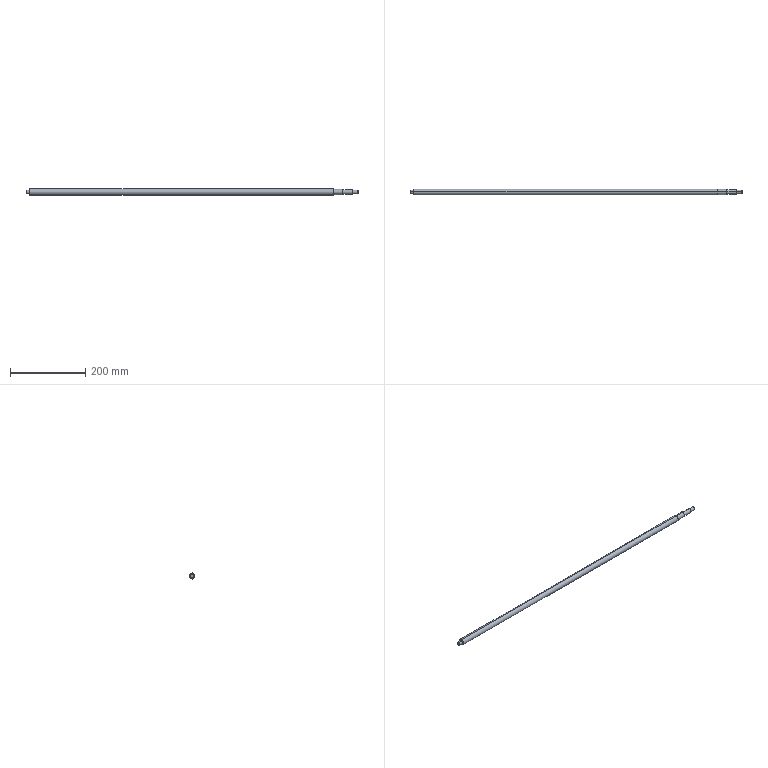Part | STEP file | Lead screw 16V1.201001 | 1 solid | 20 faces | box 882 x 16 x 16 mm | volume 170889 mm3 | cylinder 10 | plane 6 | cone 4 | commonest cylinder face diameters 10 x4 12 x2 14 x2 16 x2
STEP:
#1=CARTESIAN_POINT('',(0.,0.,0.));
#2=DIRECTION('',(0.,0.,1.));
#3=DIRECTION('',(1.,0.,0.));
#4=AXIS2_PLACEMENT_3D('',#1,#2,#3);
#5=CARTESIAN_POINT('',(817.,0.,-8.));
#6=VERTEX_POINT('',#5);
#7=CARTESIAN_POINT('',(817.,0.,8.));
#8=VERTEX_POINT('',#7);
#9=CARTESIAN_POINT('',(817.,0.,0.));
#10=DIRECTION('',(1.,0.,0.));
#11=DIRECTION('',(0.,0.,-1.));
#12=AXIS2_PLACEMENT_3D('',#9,#10,#11);
#13=CIRCLE('',#12,8.);
#14=CARTESIAN_POINT('',(830.,0.,0.));
#15=DIRECTION('',(-1.,0.,0.));
#16=DIRECTION('',(0.,0.,1.));
#17=AXIS2_PLACEMENT_3D('',#14,#15,#16);
#18=CYLINDRICAL_SURFACE('',#17,8.);
#19=CARTESIAN_POINT('',(3.142,13.));
#20=DIRECTION('',(-1.,0.));
#21=VECTOR('',#20,1.);
#22=LINE('',#19,#21);
#23=(GEOMETRIC_REPRESENTATION_CONTEXT(2)PARAMETRIC_REPRESENTATION_CONTEXT()REPRESENTATION_CONTEXT('',''));
#24=DEFINITIONAL_REPRESENTATION('',(#22),#23);
#25=PCURVE('',#18,#24);
#26=CARTESIAN_POINT('',(817.,0.,0.));
#27=DIRECTION('',(1.,0.,0.));
#28=DIRECTION('',(0.,0.,-1.));
#29=AXIS2_PLACEMENT_3D('',#26,#27,#28);
#30=PLANE('',#29);
#31=CARTESIAN_POINT('',(0.,0.));
#32=DIRECTION('',(1.,0.));
#33=AXIS2_PLACEMENT_2D('',#31,#32);
#34=CIRCLE('',#33,8.);
#35=(GEOMETRIC_REPRESENTATION_CONTEXT(2)PARAMETRIC_REPRESENTATION_CONTEXT()REPRESENTATION_CONTEXT('',''));
#36=DEFINITIONAL_REPRESENTATION('',(#34),#35);
#37=PCURVE('',#30,#36);
#38=SURFACE_CURVE('',#13,(#25,#37),.PCURVE_S1.);
#39=EDGE_CURVE('',#6,#8,#38,.T.);
#40=ORIENTED_EDGE('',*,*,#39,.F.);
#41=CARTESIAN_POINT('',(10.,0.,-8.));
#42=VERTEX_POINT('',#41);
#43=CARTESIAN_POINT('',(830.,0.,-8.));
#44=DIRECTION('',(-1.,0.,0.));
#45=VECTOR('',#44,1.);
#46=LINE('',#43,#45);
#47=CARTESIAN_POINT('',(3.142,0.));
#48=DIRECTION('',(0.,1.));
#49=VECTOR('',#48,1.);
#50=LINE('',#47,#49);
#51=(GEOMETRIC_REPRESENTATION_CONTEXT(2)PARAMETRIC_REPRESENTATION_CONTEXT()REPRESENTATION_CONTEXT('',''));
#52=DEFINITIONAL_REPRESENTATION('',(#50),#51);
#53=PCURVE('',#18,#52);
#54=CARTESIAN_POINT('',(830.,0.,0.));
#55=DIRECTION('',(-1.,0.,0.));
#56=DIRECTION('',(0.,0.,1.));
#57=AXIS2_PLACEMENT_3D('',#54,#55,#56);
#58=CYLINDRICAL_SURFACE('',#57,8.);
#59=CARTESIAN_POINT('',(3.142,0.));
#60=DIRECTION('',(0.,1.));
#61=VECTOR('',#60,1.);
#62=LINE('',#59,#61);
#63=(GEOMETRIC_REPRESENTATION_CONTEXT(2)PARAMETRIC_REPRESENTATION_CONTEXT()REPRESENTATION_CONTEXT('',''));
#64=DEFINITIONAL_REPRESENTATION('',(#62),#63);
#65=PCURVE('',#58,#64);
#66=SURFACE_CURVE('',#46,(#53,#65),.PCURVE_S1.);
#67=EDGE_CURVE('',#6,#42,#66,.T.);
#68=ORIENTED_EDGE('',*,*,#67,.T.);
#69=CARTESIAN_POINT('',(10.,0.,8.));
#70=VERTEX_POINT('',#69);
#71=CARTESIAN_POINT('',(10.,0.,0.));
#72=DIRECTION('',(1.,0.,0.));
#73=DIRECTION('',(0.,0.,-1.));
#74=AXIS2_PLACEMENT_3D('',#71,#72,#73);
#75=CIRCLE('',#74,8.);
#76=CARTESIAN_POINT('',(3.142,820.));
#77=DIRECTION('',(-1.,0.));
#78=VECTOR('',#77,1.);
#79=LINE('',#76,#78);
#80=(GEOMETRIC_REPRESENTATION_CONTEXT(2)PARAMETRIC_REPRESENTATION_CONTEXT()REPRESENTATION_CONTEXT('',''));
#81=DEFINITIONAL_REPRESENTATION('',(#79),#80);
#82=PCURVE('',#18,#81);
#83=CARTESIAN_POINT('',(10.,0.,0.));
#84=DIRECTION('',(1.,0.,0.));
#85=DIRECTION('',(0.,0.,-1.));
#86=AXIS2_PLACEMENT_3D('',#83,#84,#85);
#87=PLANE('',#86);
#88=CARTESIAN_POINT('',(0.,0.));
#89=DIRECTION('',(1.,0.));
#90=AXIS2_PLACEMENT_2D('',#88,#89);
#91=CIRCLE('',#90,8.);
#92=(GEOMETRIC_REPRESENTATION_CONTEXT(2)PARAMETRIC_REPRESENTATION_CONTEXT()REPRESENTATION_CONTEXT('',''));
#93=DEFINITIONAL_REPRESENTATION('',(#91),#92);
#94=PCURVE('',#87,#93);
#95=SURFACE_CURVE('',#75,(#82,#94),.PCURVE_S1.);
#96=EDGE_CURVE('',#42,#70,#95,.T.);
#97=ORIENTED_EDGE('',*,*,#96,.T.);
#98=CARTESIAN_POINT('',(830.,0.,8.));
#99=DIRECTION('',(-1.,0.,0.));
#100=VECTOR('',#99,1.);
#101=LINE('',#98,#100);
#102=CARTESIAN_POINT('',(0.,0.));
#103=DIRECTION('',(0.,1.));
#104=VECTOR('',#103,1.);
#105=LINE('',#102,#104);
#106=(GEOMETRIC_REPRESENTATION_CONTEXT(2)PARAMETRIC_REPRESENTATION_CONTEXT()REPRESENTATION_CONTEXT('',''));
#107=DEFINITIONAL_REPRESENTATION('',(#105),#106);
#108=PCURVE('',#18,#107);
#109=CARTESIAN_POINT('',(6.283,0.));
#110=DIRECTION('',(0.,1.));
#111=VECTOR('',#110,1.);
#112=LINE('',#109,#111);
#113=(GEOMETRIC_REPRESENTATION_CONTEXT(2)PARAMETRIC_REPRESENTATION_CONTEXT()REPRESENTATION_CONTEXT('',''));
#114=DEFINITIONAL_REPRESENTATION('',(#112),#113);
#115=PCURVE('',#58,#114);
#116=SURFACE_CURVE('',#101,(#108,#115),.PCURVE_S1.);
#117=EDGE_CURVE('',#8,#70,#116,.T.);
#118=ORIENTED_EDGE('',*,*,#117,.F.);
#119=EDGE_LOOP('',(#40,#68,#97,#118));
#120=FACE_BOUND('',#119,.T.);
#121=ADVANCED_FACE('',(#120),#18,.T.);
#122=CARTESIAN_POINT('',(10.,0.,-5.));
#123=VERTEX_POINT('',#122);
#124=CARTESIAN_POINT('',(10.,0.,5.));
#125=VERTEX_POINT('',#124);
#126=CARTESIAN_POINT('',(10.,0.,0.));
#127=DIRECTION('',(1.,0.,0.));
#128=DIRECTION('',(0.,0.,-1.));
#129=AXIS2_PLACEMENT_3D('',#126,#127,#128);
#130=CIRCLE('',#129,5.);
#131=CARTESIAN_POINT('',(10.,0.,0.));
#132=DIRECTION('',(-1.,0.,0.));
#133=DIRECTION('',(0.,0.,1.));
#134=AXIS2_PLACEMENT_3D('',#131,#132,#133);
#135=CYLINDRICAL_SURFACE('',#134,5.);
#136=CARTESIAN_POINT('',(3.142,0.));
#137=DIRECTION('',(-1.,0.));
#138=VECTOR('',#137,1.);
#139=LINE('',#136,#138);
#140=(GEOMETRIC_REPRESENTATION_CONTEXT(2)PARAMETRIC_REPRESENTATION_CONTEXT()REPRESENTATION_CONTEXT('',''));
#141=DEFINITIONAL_REPRESENTATION('',(#139),#140);
#142=PCURVE('',#135,#141);
#143=CARTESIAN_POINT('',(0.,0.));
#144=DIRECTION('',(1.,0.));
#145=AXIS2_PLACEMENT_2D('',#143,#144);
#146=CIRCLE('',#145,5.);
#147=(GEOMETRIC_REPRESENTATION_CONTEXT(2)PARAMETRIC_REPRESENTATION_CONTEXT()REPRESENTATION_CONTEXT('',''));
#148=DEFINITIONAL_REPRESENTATION('',(#146),#147);
#149=PCURVE('',#87,#148);
#150=SURFACE_CURVE('',#130,(#142,#149),.PCURVE_S1.);
#151=EDGE_CURVE('',#123,#125,#150,.T.);
#152=ORIENTED_EDGE('',*,*,#151,.F.);
#153=CARTESIAN_POINT('',(0.5,0.,-5.));
#154=VERTEX_POINT('',#153);
#155=CARTESIAN_POINT('',(10.,0.,-5.));
#156=DIRECTION('',(-1.,0.,0.));
#157=VECTOR('',#156,1.);
#158=LINE('',#155,#157);
#159=CARTESIAN_POINT('',(3.142,0.));
#160=DIRECTION('',(0.,1.));
#161=VECTOR('',#160,1.);
#162=LINE('',#159,#161);
#163=(GEOMETRIC_REPRESENTATION_CONTEXT(2)PARAMETRIC_REPRESENTATION_CONTEXT()REPRESENTATION_CONTEXT('',''));
#164=DEFINITIONAL_REPRESENTATION('',(#162),#163);
#165=PCURVE('',#135,#164);
#166=CARTESIAN_POINT('',(10.,0.,0.));
#167=DIRECTION('',(-1.,0.,0.));
#168=DIRECTION('',(0.,0.,1.));
#169=AXIS2_PLACEMENT_3D('',#166,#167,#168);
#170=CYLINDRICAL_SURFACE('',#169,5.);
#171=CARTESIAN_POINT('',(3.142,0.));
#172=DIRECTION('',(0.,1.));
#173=VECTOR('',#172,1.);
#174=LINE('',#171,#173);
#175=(GEOMETRIC_REPRESENTATION_CONTEXT(2)PARAMETRIC_REPRESENTATION_CONTEXT()REPRESENTATION_CONTEXT('',''));
#176=DEFINITIONAL_REPRESENTATION('',(#174),#175);
#177=PCURVE('',#170,#176);
#178=SURFACE_CURVE('',#158,(#165,#177),.PCURVE_S1.);
#179=EDGE_CURVE('',#123,#154,#178,.T.);
#180=ORIENTED_EDGE('',*,*,#179,.T.);
#181=CARTESIAN_POINT('',(0.5,0.,5.));
#182=VERTEX_POINT('',#181);
#183=CARTESIAN_POINT('',(0.5,0.,0.));
#184=DIRECTION('',(1.,0.,0.));
#185=DIRECTION('',(0.,0.,-1.));
#186=AXIS2_PLACEMENT_3D('',#183,#184,#185);
#187=CIRCLE('',#186,5.);
#188=CARTESIAN_POINT('',(3.142,9.5));
#189=DIRECTION('',(-1.,0.));
#190=VECTOR('',#189,1.);
#191=LINE('',#188,#190);
#192=(GEOMETRIC_REPRESENTATION_CONTEXT(2)PARAMETRIC_REPRESENTATION_CONTEXT()REPRESENTATION_CONTEXT('',''));
#193=DEFINITIONAL_REPRESENTATION('',(#191),#192);
#194=PCURVE('',#135,#193);
#195=CARTESIAN_POINT('',(0.5,0.,0.));
#196=DIRECTION('',(1.,0.,0.));
#197=DIRECTION('',(0.,0.,-1.));
#198=AXIS2_PLACEMENT_3D('',#195,#196,#197);
#199=CONICAL_SURFACE('',#198,5.,0.7854);
#200=CARTESIAN_POINT('',(0.,0.));
#201=DIRECTION('',(1.,0.));
#202=VECTOR('',#201,1.);
#203=LINE('',#200,#202);
#204=(GEOMETRIC_REPRESENTATION_CONTEXT(2)PARAMETRIC_REPRESENTATION_CONTEXT()REPRESENTATION_CONTEXT('',''));
#205=DEFINITIONAL_REPRESENTATION('',(#203),#204);
#206=PCURVE('',#199,#205);
#207=SURFACE_CURVE('',#187,(#194,#206),.PCURVE_S1.);
#208=EDGE_CURVE('',#154,#182,#207,.T.);
#209=ORIENTED_EDGE('',*,*,#208,.T.);
#210=CARTESIAN_POINT('',(10.,0.,5.));
#211=DIRECTION('',(-1.,0.,0.));
#212=VECTOR('',#211,1.);
#213=LINE('',#210,#212);
#214=CARTESIAN_POINT('',(0.,0.));
#215=DIRECTION('',(0.,1.));
#216=VECTOR('',#215,1.);
#217=LINE('',#214,#216);
#218=(GEOMETRIC_REPRESENTATION_CONTEXT(2)PARAMETRIC_REPRESENTATION_CONTEXT()REPRESENTATION_CONTEXT('',''));
#219=DEFINITIONAL_REPRESENTATION('',(#217),#218);
#220=PCURVE('',#135,#219);
#221=CARTESIAN_POINT('',(6.283,0.));
#222=DIRECTION('',(0.,1.));
#223=VECTOR('',#222,1.);
#224=LINE('',#221,#223);
#225=(GEOMETRIC_REPRESENTATION_CONTEXT(2)PARAMETRIC_REPRESENTATION_CONTEXT()REPRESENTATION_CONTEXT('',''));
#226=DEFINITIONAL_REPRESENTATION('',(#224),#225);
#227=PCURVE('',#170,#226);
#228=SURFACE_CURVE('',#213,(#220,#227),.PCURVE_S1.);
#229=EDGE_CURVE('',#125,#182,#228,.T.);
#230=ORIENTED_EDGE('',*,*,#229,.F.);
#231=EDGE_LOOP('',(#152,#180,#209,#230));
#232=FACE_BOUND('',#231,.T.);
#233=ADVANCED_FACE('',(#232),#135,.T.);
#234=CARTESIAN_POINT('',(0.,0.,4.5));
#235=VERTEX_POINT('',#234);
#236=CARTESIAN_POINT('',(0.,0.,-4.5));
#237=VERTEX_POINT('',#236);
#238=CARTESIAN_POINT('',(0.,0.,0.));
#239=DIRECTION('',(-1.,0.,0.));
#240=DIRECTION('',(0.,0.,-1.));
#241=AXIS2_PLACEMENT_3D('',#238,#239,#240);
#242=CIRCLE('',#241,4.5);
#243=CARTESIAN_POINT('',(6.283,-0.5));
#244=DIRECTION('',(-1.,0.));
#245=VECTOR('',#244,1.);
#246=LINE('',#243,#245);
#247=(GEOMETRIC_REPRESENTATION_CONTEXT(2)PARAMETRIC_REPRESENTATION_CONTEXT()REPRESENTATION_CONTEXT('',''));
#248=DEFINITIONAL_REPRESENTATION('',(#246),#247);
#249=PCURVE('',#199,#248);
#250=CARTESIAN_POINT('',(0.,0.,0.));
#251=DIRECTION('',(1.,0.,0.));
#252=DIRECTION('',(0.,0.,-1.));
#253=AXIS2_PLACEMENT_3D('',#250,#251,#252);
#254=PLANE('',#253);
#255=CARTESIAN_POINT('',(4.5,0.));
#256=CARTESIAN_POINT('',(4.5,-7.794));
#257=CARTESIAN_POINT('',(-2.25,-3.897));
#258=CARTESIAN_POINT('',(-9.,0.));
#259=CARTESIAN_POINT('',(-2.25,3.897));
#260=CARTESIAN_POINT('',(4.5,7.794));
#261=CARTESIAN_POINT('',(4.5,0.));
#262=(BOUNDED_CURVE()B_SPLINE_CURVE(2,(#255,#256,#257,#258,#259,#260,#261),.UNSPECIFIED.,.T.,.F.)B_SPLINE_CURVE_WITH_KNOTS((1,2,2,2,2,1),(-2.094,0.,2.094,4.189,6.283,8.378),.UNSPECIFIED.)CURVE()GEOMETRIC_REPRESENTATION_ITEM()RATIONAL_B_SPLINE_CURVE((1.,0.5,1.,0.5,1.,0.5,1.))REPRESENTATION_ITEM(''));
#263=(GEOMETRIC_REPRESENTATION_CONTEXT(2)PARAMETRIC_REPRESENTATION_CONTEXT()REPRESENTATION_CONTEXT('',''));
#264=DEFINITIONAL_REPRESENTATION('',(#262),#263);
#265=PCURVE('',#254,#264);
#266=SURFACE_CURVE('',#242,(#249,#265),.PCURVE_S1.);
#267=EDGE_CURVE('',#235,#237,#266,.T.);
#268=ORIENTED_EDGE('',*,*,#267,.F.);
#269=CARTESIAN_POINT('',(0.5,0.,5.));
#270=DIRECTION('',(0.7071,0.,0.7071));
#271=VECTOR('',#270,1.);
#272=LINE('',#269,#271);
#273=CARTESIAN_POINT('',(3.142,0.));
#274=DIRECTION('',(0.,1.));
#275=VECTOR('',#274,1.);
#276=LINE('',#273,#275);
#277=(GEOMETRIC_REPRESENTATION_CONTEXT(2)PARAMETRIC_REPRESENTATION_CONTEXT()REPRESENTATION_CONTEXT('',''));
#278=DEFINITIONAL_REPRESENTATION('',(#276),#277);
#279=PCURVE('',#199,#278);
#280=CARTESIAN_POINT('',(0.5,0.,0.));
#281=DIRECTION('',(1.,0.,0.));
#282=DIRECTION('',(0.,0.,-1.));
#283=AXIS2_PLACEMENT_3D('',#280,#281,#282);
#284=CONICAL_SURFACE('',#283,5.,0.7854);
#285=CARTESIAN_POINT('',(3.142,0.));
#286=DIRECTION('',(0.,1.));
#287=VECTOR('',#286,1.);
#288=LINE('',#285,#287);
#289=(GEOMETRIC_REPRESENTATION_CONTEXT(2)PARAMETRIC_REPRESENTATION_CONTEXT()REPRESENTATION_CONTEXT('',''));
#290=DEFINITIONAL_REPRESENTATION('',(#288),#289);
#291=PCURVE('',#284,#290);
#292=SURFACE_CURVE('',#272,(#279,#291),.PCURVE_S1.);
#293=EDGE_CURVE('',#235,#182,#292,.T.);
#294=ORIENTED_EDGE('',*,*,#293,.T.);
#295=ORIENTED_EDGE('',*,*,#208,.F.);
#296=CARTESIAN_POINT('',(0.5,0.,-5.));
#297=DIRECTION('',(0.7071,0.,-0.7071));
#298=VECTOR('',#297,1.);
#299=LINE('',#296,#298);
#300=CARTESIAN_POINT('',(0.,0.));
#301=DIRECTION('',(0.,1.));
#302=VECTOR('',#301,1.);
#303=LINE('',#300,#302);
#304=(GEOMETRIC_REPRESENTATION_CONTEXT(2)PARAMETRIC_REPRESENTATION_CONTEXT()REPRESENTATION_CONTEXT('',''));
#305=DEFINITIONAL_REPRESENTATION('',(#303),#304);
#306=PCURVE('',#199,#305);
#307=CARTESIAN_POINT('',(6.283,0.));
#308=DIRECTION('',(0.,1.));
#309=VECTOR('',#308,1.);
#310=LINE('',#307,#309);
#311=(GEOMETRIC_REPRESENTATION_CONTEXT(2)PARAMETRIC_REPRESENTATION_CONTEXT()REPRESENTATION_CONTEXT('',''));
#312=DEFINITIONAL_REPRESENTATION('',(#310),#311);
#313=PCURVE('',#284,#312);
#314=SURFACE_CURVE('',#299,(#306,#313),.PCURVE_S1.);
#315=EDGE_CURVE('',#237,#154,#314,.T.);
#316=ORIENTED_EDGE('',*,*,#315,.F.);
#317=EDGE_LOOP('',(#268,#294,#295,#316));
#318=FACE_BOUND('',#317,.T.);
#319=ADVANCED_FACE('',(#318),#199,.T.);
#320=CARTESIAN_POINT('',(817.,0.,-7.));
#321=VERTEX_POINT('',#320);
#322=CARTESIAN_POINT('',(817.,0.,7.));
#323=VERTEX_POINT('',#322);
#324=CARTESIAN_POINT('',(817.,0.,0.));
#325=DIRECTION('',(1.,0.,0.));
#326=DIRECTION('',(0.,0.,-1.));
#327=AXIS2_PLACEMENT_3D('',#324,#325,#326);
#328=CIRCLE('',#327,7.);
#329=CARTESIAN_POINT('',(817.,0.,0.));
#330=DIRECTION('',(1.,0.,0.));
#331=DIRECTION('',(0.,0.,-1.));
#332=AXIS2_PLACEMENT_3D('',#329,#330,#331);
#333=CYLINDRICAL_SURFACE('',#332,7.);
#334=CARTESIAN_POINT('',(0.,0.));
#335=DIRECTION('',(1.,0.));
#336=VECTOR('',#335,1.);
#337=LINE('',#334,#336);
#338=(GEOMETRIC_REPRESENTATION_CONTEXT(2)PARAMETRIC_REPRESENTATION_CONTEXT()REPRESENTATION_CONTEXT('',''));
#339=DEFINITIONAL_REPRESENTATION('',(#337),#338);
#340=PCURVE('',#333,#339);
#341=CARTESIAN_POINT('',(0.,0.));
#342=DIRECTION('',(1.,0.));
#343=AXIS2_PLACEMENT_2D('',#341,#342);
#344=CIRCLE('',#343,7.);
#345=(GEOMETRIC_REPRESENTATION_CONTEXT(2)PARAMETRIC_REPRESENTATION_CONTEXT()REPRESENTATION_CONTEXT('',''));
#346=DEFINITIONAL_REPRESENTATION('',(#344),#345);
#347=PCURVE('',#30,#346);
#348=SURFACE_CURVE('',#328,(#340,#347),.PCURVE_S1.);
#349=EDGE_CURVE('',#321,#323,#348,.T.);
#350=ORIENTED_EDGE('',*,*,#349,.T.);
#351=CARTESIAN_POINT('',(842.,0.,7.));
#352=VERTEX_POINT('',#351);
#353=CARTESIAN_POINT('',(817.,0.,7.));
#354=DIRECTION('',(1.,0.,0.));
#355=VECTOR('',#354,1.);
#356=LINE('',#353,#355);
#357=CARTESIAN_POINT('',(3.142,0.));
#358=DIRECTION('',(0.,1.));
#359=VECTOR('',#358,1.);
#360=LINE('',#357,#359);
#361=(GEOMETRIC_REPRESENTATION_CONTEXT(2)PARAMETRIC_REPRESENTATION_CONTEXT()REPRESENTATION_CONTEXT('',''));
#362=DEFINITIONAL_REPRESENTATION('',(#360),#361);
#363=PCURVE('',#333,#362);
#364=CARTESIAN_POINT('',(817.,0.,0.));
#365=DIRECTION('',(1.,0.,0.));
#366=DIRECTION('',(0.,0.,-1.));
#367=AXIS2_PLACEMENT_3D('',#364,#365,#366);
#368=CYLINDRICAL_SURFACE('',#367,7.);
#369=CARTESIAN_POINT('',(3.142,0.));
#370=DIRECTION('',(0.,1.));
#371=VECTOR('',#370,1.);
#372=LINE('',#369,#371);
#373=(GEOMETRIC_REPRESENTATION_CONTEXT(2)PARAMETRIC_REPRESENTATION_CONTEXT()REPRESENTATION_CONTEXT('',''));
#374=DEFINITIONAL_REPRESENTATION('',(#372),#373);
#375=PCURVE('',#368,#374);
#376=SURFACE_CURVE('',#356,(#363,#375),.PCURVE_S1.);
#377=EDGE_CURVE('',#323,#352,#376,.T.);
#378=ORIENTED_EDGE('',*,*,#377,.T.);
#379=CARTESIAN_POINT('',(842.,0.,-7.));
#380=VERTEX_POINT('',#379);
#381=CARTESIAN_POINT('',(842.,0.,0.));
#382=DIRECTION('',(1.,0.,0.));
#383=DIRECTION('',(0.,0.,-1.));
#384=AXIS2_PLACEMENT_3D('',#381,#382,#383);
#385=CIRCLE('',#384,7.);
#386=CARTESIAN_POINT('',(0.,25.));
#387=DIRECTION('',(1.,0.));
#388=VECTOR('',#387,1.);
#389=LINE('',#386,#388);
#390=(GEOMETRIC_REPRESENTATION_CONTEXT(2)PARAMETRIC_REPRESENTATION_CONTEXT()REPRESENTATION_CONTEXT('',''));
#391=DEFINITIONAL_REPRESENTATION('',(#389),#390);
#392=PCURVE('',#333,#391);
#393=CARTESIAN_POINT('',(842.,0.,0.));
#394=DIRECTION('',(1.,0.,0.));
#395=DIRECTION('',(0.,0.,-1.));
#396=AXIS2_PLACEMENT_3D('',#393,#394,#395);
#397=PLANE('',#396);
#398=CARTESIAN_POINT('',(0.,0.));
#399=DIRECTION('',(1.,0.));
#400=AXIS2_PLACEMENT_2D('',#398,#399);
#401=CIRCLE('',#400,7.);
#402=(GEOMETRIC_REPRESENTATION_CONTEXT(2)PARAMETRIC_REPRESENTATION_CONTEXT()REPRESENTATION_CONTEXT('',''));
#403=DEFINITIONAL_REPRESENTATION('',(#401),#402);
#404=PCURVE('',#397,#403);
#405=SURFACE_CURVE('',#385,(#392,#404),.PCURVE_S1.);
#406=EDGE_CURVE('',#380,#352,#405,.T.);
#407=ORIENTED_EDGE('',*,*,#406,.F.);
#408=CARTESIAN_POINT('',(817.,0.,-7.));
#409=DIRECTION('',(1.,0.,0.));
#410=VECTOR('',#409,1.);
#411=LINE('',#408,#410);
#412=CARTESIAN_POINT('',(0.,0.));
#413=DIRECTION('',(0.,1.));
#414=VECTOR('',#413,1.);
#415=LINE('',#412,#414);
#416=(GEOMETRIC_REPRESENTATION_CONTEXT(2)PARAMETRIC_REPRESENTATION_CONTEXT()REPRESENTATION_CONTEXT('',''));
#417=DEFINITIONAL_REPRESENTATION('',(#415),#416);
#418=PCURVE('',#333,#417);
#419=CARTESIAN_POINT('',(6.283,0.));
#420=DIRECTION('',(0.,1.));
#421=VECTOR('',#420,1.);
#422=LINE('',#419,#421);
#423=(GEOMETRIC_REPRESENTATION_CONTEXT(2)PARAMETRIC_REPRESENTATION_CONTEXT()REPRESENTATION_CONTEXT('',''));
#424=DEFINITIONAL_REPRESENTATION('',(#422),#423);
#425=PCURVE('',#368,#424);
#426=SURFACE_CURVE('',#411,(#418,#425),.PCURVE_S1.);
#427=EDGE_CURVE('',#321,#380,#426,.T.);
#428=ORIENTED_EDGE('',*,*,#427,.F.);
#429=EDGE_LOOP('',(#350,#378,#407,#428));
#430=FACE_BOUND('',#429,.T.);
#431=ADVANCED_FACE('',(#430),#333,.T.);
#432=CARTESIAN_POINT('',(882.,0.,-4.5));
#433=VERTEX_POINT('',#432);
#434=CARTESIAN_POINT('',(882.,0.,4.5));
#435=VERTEX_POINT('',#434);
#436=CARTESIAN_POINT('',(882.,0.,0.));
#437=DIRECTION('',(1.,0.,0.));
#438=DIRECTION('',(0.,0.,-1.));
#439=AXIS2_PLACEMENT_3D('',#436,#437,#438);
#440=CIRCLE('',#439,4.5);
#441=CARTESIAN_POINT('',(882.,0.,0.));
#442=DIRECTION('',(-1.,0.,0.));
#443=DIRECTION('',(0.,0.,1.));
#444=AXIS2_PLACEMENT_3D('',#441,#442,#443);
#445=CONICAL_SURFACE('',#444,4.5,0.7854);
#446=CARTESIAN_POINT('',(3.142,0.));
#447=DIRECTION('',(-1.,0.));
#448=VECTOR('',#447,1.);
#449=LINE('',#446,#448);
#450=(GEOMETRIC_REPRESENTATION_CONTEXT(2)PARAMETRIC_REPRESENTATION_CONTEXT()REPRESENTATION_CONTEXT('',''));
#451=DEFINITIONAL_REPRESENTATION('',(#449),#450);
#452=PCURVE('',#445,#451);
#453=CARTESIAN_POINT('',(882.,0.,0.));
#454=DIRECTION('',(1.,0.,0.));
#455=DIRECTION('',(0.,0.,-1.));
#456=AXIS2_PLACEMENT_3D('',#453,#454,#455);
#457=PLANE('',#456);
#458=CARTESIAN_POINT('',(0.,0.));
#459=DIRECTION('',(1.,0.));
#460=AXIS2_PLACEMENT_2D('',#458,#459);
#461=CIRCLE('',#460,4.5);
#462=(GEOMETRIC_REPRESENTATION_CONTEXT(2)PARAMETRIC_REPRESENTATION_CONTEXT()REPRESENTATION_CONTEXT('',''));
#463=DEFINITIONAL_REPRESENTATION('',(#461),#462);
#464=PCURVE('',#457,#463);
#465=SURFACE_CURVE('',#440,(#452,#464),.PCURVE_S1.);
#466=EDGE_CURVE('',#433,#435,#465,.T.);
#467=ORIENTED_EDGE('',*,*,#466,.F.);
#468=CARTESIAN_POINT('',(881.5,0.,-5.));
#469=VERTEX_POINT('',#468);
#470=CARTESIAN_POINT('',(882.,0.,-4.5));
#471=DIRECTION('',(-0.7071,0.,-0.7071));
#472=VECTOR('',#471,1.);
#473=LINE('',#470,#472);
#474=CARTESIAN_POINT('',(3.142,0.));
#475=DIRECTION('',(0.,1.));
#476=VECTOR('',#475,1.);
#477=LINE('',#474,#476);
#478=(GEOMETRIC_REPRESENTATION_CONTEXT(2)PARAMETRIC_REPRESENTATION_CONTEXT()REPRESENTATION_CONTEXT('',''));
#479=DEFINITIONAL_REPRESENTATION('',(#477),#478);
#480=PCURVE('',#445,#479);
#481=CARTESIAN_POINT('',(882.,0.,0.));
#482=DIRECTION('',(-1.,0.,0.));
#483=DIRECTION('',(0.,0.,1.));
#484=AXIS2_PLACEMENT_3D('',#481,#482,#483);
#485=CONICAL_SURFACE('',#484,4.5,0.7854);
#486=CARTESIAN_POINT('',(3.142,0.));
#487=DIRECTION('',(0.,1.));
#488=VECTOR('',#487,1.);
#489=LINE('',#486,#488);
#490=(GEOMETRIC_REPRESENTATION_CONTEXT(2)PARAMETRIC_REPRESENTATION_CONTEXT()REPRESENTATION_CONTEXT('',''));
#491=DEFINITIONAL_REPRESENTATION('',(#489),#490);
#492=PCURVE('',#485,#491);
#493=SURFACE_CURVE('',#473,(#480,#492),.PCURVE_S1.);
#494=EDGE_CURVE('',#433,#469,#493,.T.);
#495=ORIENTED_EDGE('',*,*,#494,.T.);
#496=CARTESIAN_POINT('',(881.5,0.,5.));
#497=VERTEX_POINT('',#496);
#498=CARTESIAN_POINT('',(881.5,0.,0.));
#499=DIRECTION('',(-1.,0.,0.));
#500=DIRECTION('',(0.,0.,-1.));
#501=AXIS2_PLACEMENT_3D('',#498,#499,#500);
#502=CIRCLE('',#501,5.);
#503=CARTESIAN_POINT('',(-3.142,0.5));
#504=DIRECTION('',(1.,0.));
#505=VECTOR('',#504,1.);
#506=LINE('',#503,#505);
#507=(GEOMETRIC_REPRESENTATION_CONTEXT(2)PARAMETRIC_REPRESENTATION_CONTEXT()REPRESENTATION_CONTEXT('',''));
#508=DEFINITIONAL_REPRESENTATION('',(#506),#507);
#509=PCURVE('',#445,#508);
#510=CARTESIAN_POINT('',(882.,0.,0.));
#511=DIRECTION('',(-1.,0.,0.));
#512=DIRECTION('',(0.,0.,1.));
#513=AXIS2_PLACEMENT_3D('',#510,#511,#512);
#514=CYLINDRICAL_SURFACE('',#513,5.);
#515=CARTESIAN_POINT('',(-3.142,0.5));
#516=DIRECTION('',(1.,0.));
#517=VECTOR('',#516,1.);
#518=LINE('',#515,#517);
#519=(GEOMETRIC_REPRESENTATION_CONTEXT(2)PARAMETRIC_REPRESENTATION_CONTEXT()REPRESENTATION_CONTEXT('',''));
#520=DEFINITIONAL_REPRESENTATION('',(#518),#519);
#521=PCURVE('',#514,#520);
#522=SURFACE_CURVE('',#502,(#509,#521),.PCURVE_S1.);
#523=EDGE_CURVE('',#497,#469,#522,.T.);
#524=ORIENTED_EDGE('',*,*,#523,.F.);
#525=CARTESIAN_POINT('',(882.,0.,4.5));
#526=DIRECTION('',(-0.7071,0.,0.7071));
#527=VECTOR('',#526,1.);
#528=LINE('',#525,#527);
#529=CARTESIAN_POINT('',(0.,0.));
#530=DIRECTION('',(0.,1.));
#531=VECTOR('',#530,1.);
#532=LINE('',#529,#531);
#533=(GEOMETRIC_REPRESENTATION_CONTEXT(2)PARAMETRIC_REPRESENTATION_CONTEXT()REPRESENTATION_CONTEXT('',''));
#534=DEFINITIONAL_REPRESENTATION('',(#532),#533);
#535=PCURVE('',#445,#534);
#536=CARTESIAN_POINT('',(6.283,0.));
#537=DIRECTION('',(0.,1.));
#538=VECTOR('',#537,1.);
#539=LINE('',#536,#538);
#540=(GEOMETRIC_REPRESENTATION_CONTEXT(2)PARAMETRIC_REPRESENTATION_CONTEXT()REPRESENTATION_CONTEXT('',''));
#541=DEFINITIONAL_REPRESENTATION('',(#539),#540);
#542=PCURVE('',#485,#541);
#543=SURFACE_CURVE('',#528,(#535,#542),.PCURVE_S1.);
#544=EDGE_CURVE('',#435,#497,#543,.T.);
#545=ORIENTED_EDGE('',*,*,#544,.F.);
#546=EDGE_LOOP('',(#467,#495,#524,#545));
#547=FACE_BOUND('',#546,.T.);
#548=ADVANCED_FACE('',(#547),#445,.T.);
#549=ORIENTED_EDGE('',*,*,#523,.T.);
#550=CARTESIAN_POINT('',(867.,0.,-5.));
#551=VERTEX_POINT('',#550);
#552=CARTESIAN_POINT('',(882.,0.,-5.));
#553=DIRECTION('',(-1.,0.,0.));
#554=VECTOR('',#553,1.);
#555=LINE('',#552,#554);
#556=CARTESIAN_POINT('',(3.142,0.));
#557=DIRECTION('',(0.,1.));
#558=VECTOR('',#557,1.);
#559=LINE('',#556,#558);
#560=(GEOMETRIC_REPRESENTATION_CONTEXT(2)PARAMETRIC_REPRESENTATION_CONTEXT()REPRESENTATION_CONTEXT('',''));
#561=DEFINITIONAL_REPRESENTATION('',(#559),#560);
#562=PCURVE('',#514,#561);
#563=CARTESIAN_POINT('',(882.,0.,0.));
#564=DIRECTION('',(-1.,0.,0.));
#565=DIRECTION('',(0.,0.,1.));
#566=AXIS2_PLACEMENT_3D('',#563,#564,#565);
#567=CYLINDRICAL_SURFACE('',#566,5.);
#568=CARTESIAN_POINT('',(3.142,0.));
#569=DIRECTION('',(0.,1.));
#570=VECTOR('',#569,1.);
#571=LINE('',#568,#570);
#572=(GEOMETRIC_REPRESENTATION_CONTEXT(2)PARAMETRIC_REPRESENTATION_CONTEXT()REPRESENTATION_CONTEXT('',''));
#573=DEFINITIONAL_REPRESENTATION('',(#571),#572);
#574=PCURVE('',#567,#573);
#575=SURFACE_CURVE('',#555,(#562,#574),.PCURVE_S1.);
#576=EDGE_CURVE('',#469,#551,#575,.T.);
#577=ORIENTED_EDGE('',*,*,#576,.T.);
#578=CARTESIAN_POINT('',(867.,0.,5.));
#579=VERTEX_POINT('',#578);
#580=CARTESIAN_POINT('',(867.,0.,0.));
#581=DIRECTION('',(1.,0.,0.));
#582=DIRECTION('',(0.,0.,-1.));
#583=AXIS2_PLACEMENT_3D('',#580,#581,#582);
#584=CIRCLE('',#583,5.);
#585=CARTESIAN_POINT('',(3.142,15.));
#586=DIRECTION('',(-1.,0.));
#587=VECTOR('',#586,1.);
#588=LINE('',#585,#587);
#589=(GEOMETRIC_REPRESENTATION_CONTEXT(2)PARAMETRIC_REPRESENTATION_CONTEXT()REPRESENTATION_CONTEXT('',''));
#590=DEFINITIONAL_REPRESENTATION('',(#588),#589);
#591=PCURVE('',#514,#590);
#592=CARTESIAN_POINT('',(867.,0.,0.));
#593=DIRECTION('',(1.,0.,0.));
#594=DIRECTION('',(0.,0.,-1.));
#595=AXIS2_PLACEMENT_3D('',#592,#593,#594);
#596=PLANE('',#595);
#597=CARTESIAN_POINT('',(0.,0.));
#598=DIRECTION('',(1.,0.));
#599=AXIS2_PLACEMENT_2D('',#597,#598);
#600=CIRCLE('',#599,5.);
#601=(GEOMETRIC_REPRESENTATION_CONTEXT(2)PARAMETRIC_REPRESENTATION_CONTEXT()REPRESENTATION_CONTEXT('',''));
#602=DEFINITIONAL_REPRESENTATION('',(#600),#601);
#603=PCURVE('',#596,#602);
#604=SURFACE_CURVE('',#584,(#591,#603),.PCURVE_S1.);
#605=EDGE_CURVE('',#551,#579,#604,.T.);
#606=ORIENTED_EDGE('',*,*,#605,.T.);
#607=CARTESIAN_POINT('',(882.,0.,5.));
#608=DIRECTION('',(-1.,0.,0.));
#609=VECTOR('',#608,1.);
#610=LINE('',#607,#609);
#611=CARTESIAN_POINT('',(0.,0.));
#612=DIRECTION('',(0.,1.));
#613=VECTOR('',#612,1.);
#614=LINE('',#611,#613);
#615=(GEOMETRIC_REPRESENTATION_CONTEXT(2)PARAMETRIC_REPRESENTATION_CONTEXT()REPRESENTATION_CONTEXT('',''));
#616=DEFINITIONAL_REPRESENTATION('',(#614),#615);
#617=PCURVE('',#514,#616);
#618=CARTESIAN_POINT('',(6.283,0.));
#619=DIRECTION('',(0.,1.));
#620=VECTOR('',#619,1.);
#621=LINE('',#618,#620);
#622=(GEOMETRIC_REPRESENTATION_CONTEXT(2)PARAMETRIC_REPRESENTATION_CONTEXT()REPRESENTATION_CONTEXT('',''));
#623=DEFINITIONAL_REPRESENTATION('',(#621),#622);
#624=PCURVE('',#567,#623);
#625=SURFACE_CURVE('',#610,(#617,#624),.PCURVE_S1.);
#626=EDGE_CURVE('',#497,#579,#625,.T.);
#627=ORIENTED_EDGE('',*,*,#626,.F.);
#628=EDGE_LOOP('',(#549,#577,#606,#627));
#629=FACE_BOUND('',#628,.T.);
#630=ADVANCED_FACE('',(#629),#514,.T.);
#631=CARTESIAN_POINT('',(867.,0.,-6.));
#632=VERTEX_POINT('',#631);
#633=CARTESIAN_POINT('',(867.,0.,6.));
#634=VERTEX_POINT('',#633);
#635=CARTESIAN_POINT('',(867.,0.,0.));
#636=DIRECTION('',(1.,0.,0.));
#637=DIRECTION('',(0.,0.,-1.));
#638=AXIS2_PLACEMENT_3D('',#635,#636,#637);
#639=CIRCLE('',#638,6.);
#640=CARTESIAN_POINT('',(867.,0.,0.));
#641=DIRECTION('',(-1.,0.,0.));
#642=DIRECTION('',(0.,0.,1.));
#643=AXIS2_PLACEMENT_3D('',#640,#641,#642);
#644=CYLINDRICAL_SURFACE('',#643,6.);
#645=CARTESIAN_POINT('',(3.142,0.));
#646=DIRECTION('',(-1.,0.));
#647=VECTOR('',#646,1.);
#648=LINE('',#645,#647);
#649=(GEOMETRIC_REPRESENTATION_CONTEXT(2)PARAMETRIC_REPRESENTATION_CONTEXT()REPRESENTATION_CONTEXT('',''));
#650=DEFINITIONAL_REPRESENTATION('',(#648),#649);
#651=PCURVE('',#644,#650);
#652=CARTESIAN_POINT('',(0.,0.));
#653=DIRECTION('',(1.,0.));
#654=AXIS2_PLACEMENT_2D('',#652,#653);
#655=CIRCLE('',#654,6.);
#656=(GEOMETRIC_REPRESENTATION_CONTEXT(2)PARAMETRIC_REPRESENTATION_CONTEXT()REPRESENTATION_CONTEXT('',''));
#657=DEFINITIONAL_REPRESENTATION('',(#655),#656);
#658=PCURVE('',#596,#657);
#659=SURFACE_CURVE('',#639,(#651,#658),.PCURVE_S1.);
#660=EDGE_CURVE('',#632,#634,#659,.T.);
#661=ORIENTED_EDGE('',*,*,#660,.F.);
#662=CARTESIAN_POINT('',(842.,0.,-6.));
#663=VERTEX_POINT('',#662);
#664=CARTESIAN_POINT('',(867.,0.,-6.));
#665=DIRECTION('',(-1.,0.,0.));
#666=VECTOR('',#665,1.);
#667=LINE('',#664,#666);
#668=CARTESIAN_POINT('',(3.142,0.));
#669=DIRECTION('',(0.,1.));
#670=VECTOR('',#669,1.);
#671=LINE('',#668,#670);
#672=(GEOMETRIC_REPRESENTATION_CONTEXT(2)PARAMETRIC_REPRESENTATION_CONTEXT()REPRESENTATION_CONTEXT('',''));
#673=DEFINITIONAL_REPRESENTATION('',(#671),#672);
#674=PCURVE('',#644,#673);
#675=CARTESIAN_POINT('',(867.,0.,0.));
#676=DIRECTION('',(-1.,0.,0.));
#677=DIRECTION('',(0.,0.,1.));
#678=AXIS2_PLACEMENT_3D('',#675,#676,#677);
#679=CYLINDRICAL_SURFACE('',#678,6.);
#680=CARTESIAN_POINT('',(3.142,0.));
#681=DIRECTION('',(0.,1.));
#682=VECTOR('',#681,1.);
#683=LINE('',#680,#682);
#684=(GEOMETRIC_REPRESENTATION_CONTEXT(2)PARAMETRIC_REPRESENTATION_CONTEXT()REPRESENTATION_CONTEXT('',''));
#685=DEFINITIONAL_REPRESENTATION('',(#683),#684);
#686=PCURVE('',#679,#685);
#687=SURFACE_CURVE('',#667,(#674,#686),.PCURVE_S1.);
#688=EDGE_CURVE('',#632,#663,#687,.T.);
#689=ORIENTED_EDGE('',*,*,#688,.T.);
#690=CARTESIAN_POINT('',(842.,0.,6.));
#691=VERTEX_POINT('',#690);
#692=CARTESIAN_POINT('',(842.,0.,0.));
#693=DIRECTION('',(1.,0.,0.));
#694=DIRECTION('',(0.,0.,-1.));
#695=AXIS2_PLACEMENT_3D('',#692,#693,#694);
#696=CIRCLE('',#695,6.);
#697=CARTESIAN_POINT('',(3.142,25.));
#698=DIRECTION('',(-1.,0.));
#699=VECTOR('',#698,1.);
#700=LINE('',#697,#699);
#701=(GEOMETRIC_REPRESENTATION_CONTEXT(2)PARAMETRIC_REPRESENTATION_CONTEXT()REPRESENTATION_CONTEXT('',''));
#702=DEFINITIONAL_REPRESENTATION('',(#700),#701);
#703=PCURVE('',#644,#702);
#704=CARTESIAN_POINT('',(0.,0.));
#705=DIRECTION('',(1.,0.));
#706=AXIS2_PLACEMENT_2D('',#704,#705);
#707=CIRCLE('',#706,6.);
#708=(GEOMETRIC_REPRESENTATION_CONTEXT(2)PARAMETRIC_REPRESENTATION_CONTEXT()REPRESENTATION_CONTEXT('',''));
#709=DEFINITIONAL_REPRESENTATION('',(#707),#708);
#710=PCURVE('',#397,#709);
#711=SURFACE_CURVE('',#696,(#703,#710),.PCURVE_S1.);
#712=EDGE_CURVE('',#663,#691,#711,.T.);
#713=ORIENTED_EDGE('',*,*,#712,.T.);
#714=CARTESIAN_POINT('',(867.,0.,6.));
#715=DIRECTION('',(-1.,0.,0.));
#716=VECTOR('',#715,1.);
#717=LINE('',#714,#716);
#718=CARTESIAN_POINT('',(0.,0.));
#719=DIRECTION('',(0.,1.));
#720=VECTOR('',#719,1.);
#721=LINE('',#718,#720);
#722=(GEOMETRIC_REPRESENTATION_CONTEXT(2)PARAMETRIC_REPRESENTATION_CONTEXT()REPRESENTATION_CONTEXT('',''));
#723=DEFINITIONAL_REPRESENTATION('',(#721),#722);
#724=PCURVE('',#644,#723);
#725=CARTESIAN_POINT('',(6.283,0.));
#726=DIRECTION('',(0.,1.));
#727=VECTOR('',#726,1.);
#728=LINE('',#725,#727);
#729=(GEOMETRIC_REPRESENTATION_CONTEXT(2)PARAMETRIC_REPRESENTATION_CONTEXT()REPRESENTATION_CONTEXT('',''));
#730=DEFINITIONAL_REPRESENTATION('',(#728),#729);
#731=PCURVE('',#679,#730);
#732=SURFACE_CURVE('',#717,(#724,#731),.PCURVE_S1.);
#733=EDGE_CURVE('',#634,#691,#732,.T.);
#734=ORIENTED_EDGE('',*,*,#733,.F.);
#735=EDGE_LOOP('',(#661,#689,#713,#734));
#736=FACE_BOUND('',#735,.T.);
#737=ADVANCED_FACE('',(#736),#644,.T.);
#738=CARTESIAN_POINT('',(842.,0.,0.));
#739=DIRECTION('',(1.,0.,0.));
#740=DIRECTION('',(0.,0.,-1.));
#741=AXIS2_PLACEMENT_3D('',#738,#739,#740);
#742=CIRCLE('',#741,6.);
#743=CARTESIAN_POINT('',(0.,0.));
#744=DIRECTION('',(1.,0.));
#745=AXIS2_PLACEMENT_2D('',#743,#744);
#746=CIRCLE('',#745,6.);
#747=(GEOMETRIC_REPRESENTATION_CONTEXT(2)PARAMETRIC_REPRESENTATION_CONTEXT()REPRESENTATION_CONTEXT('',''));
#748=DEFINITIONAL_REPRESENTATION('',(#746),#747);
#749=PCURVE('',#397,#748);
#750=CARTESIAN_POINT('',(9.425,25.));
#751=DIRECTION('',(-1.,0.));
#752=VECTOR('',#751,1.);
#753=LINE('',#750,#752);
#754=(GEOMETRIC_REPRESENTATION_CONTEXT(2)PARAMETRIC_REPRESENTATION_CONTEXT()REPRESENTATION_CONTEXT('',''));
#755=DEFINITIONAL_REPRESENTATION('',(#753),#754);
#756=PCURVE('',#679,#755);
#757=SURFACE_CURVE('',#742,(#749,#756),.PCURVE_S1.);
#758=EDGE_CURVE('',#691,#663,#757,.T.);
#759=ORIENTED_EDGE('',*,*,#758,.F.);
#760=ORIENTED_EDGE('',*,*,#712,.F.);
#761=EDGE_LOOP('',(#759,#760));
#762=FACE_BOUND('',#761,.T.);
#763=ORIENTED_EDGE('',*,*,#406,.T.);
#764=CARTESIAN_POINT('',(842.,0.,0.));
#765=DIRECTION('',(1.,0.,0.));
#766=DIRECTION('',(0.,0.,-1.));
#767=AXIS2_PLACEMENT_3D('',#764,#765,#766);
#768=CIRCLE('',#767,7.);
#769=CARTESIAN_POINT('',(0.,0.));
#770=DIRECTION('',(1.,0.));
#771=AXIS2_PLACEMENT_2D('',#769,#770);
#772=CIRCLE('',#771,7.);
#773=(GEOMETRIC_REPRESENTATION_CONTEXT(2)PARAMETRIC_REPRESENTATION_CONTEXT()REPRESENTATION_CONTEXT('',''));
#774=DEFINITIONAL_REPRESENTATION('',(#772),#773);
#775=PCURVE('',#397,#774);
#776=CARTESIAN_POINT('',(0.,25.));
#777=DIRECTION('',(1.,0.));
#778=VECTOR('',#777,1.);
#779=LINE('',#776,#778);
#780=(GEOMETRIC_REPRESENTATION_CONTEXT(2)PARAMETRIC_REPRESENTATION_CONTEXT()REPRESENTATION_CONTEXT('',''));
#781=DEFINITIONAL_REPRESENTATION('',(#779),#780);
#782=PCURVE('',#368,#781);
#783=SURFACE_CURVE('',#768,(#775,#782),.PCURVE_S1.);
#784=EDGE_CURVE('',#352,#380,#783,.T.);
#785=ORIENTED_EDGE('',*,*,#784,.T.);
#786=EDGE_LOOP('',(#763,#785));
#787=FACE_BOUND('',#786,.T.);
#788=ADVANCED_FACE('',(#762,#787),#397,.T.);
#789=ORIENTED_EDGE('',*,*,#688,.F.);
#790=CARTESIAN_POINT('',(867.,0.,0.));
#791=DIRECTION('',(1.,0.,0.));
#792=DIRECTION('',(0.,0.,-1.));
#793=AXIS2_PLACEMENT_3D('',#790,#791,#792);
#794=CIRCLE('',#793,6.);
#795=CARTESIAN_POINT('',(9.425,0.));
#796=DIRECTION('',(-1.,0.));
#797=VECTOR('',#796,1.);
#798=LINE('',#795,#797);
#799=(GEOMETRIC_REPRESENTATION_CONTEXT(2)PARAMETRIC_REPRESENTATION_CONTEXT()REPRESENTATION_CONTEXT('',''));
#800=DEFINITIONAL_REPRESENTATION('',(#798),#799);
#801=PCURVE('',#679,#800);
#802=CARTESIAN_POINT('',(0.,0.));
#803=DIRECTION('',(1.,0.));
#804=AXIS2_PLACEMENT_2D('',#802,#803);
#805=CIRCLE('',#804,6.);
#806=(GEOMETRIC_REPRESENTATION_CONTEXT(2)PARAMETRIC_REPRESENTATION_CONTEXT()REPRESENTATION_CONTEXT('',''));
#807=DEFINITIONAL_REPRESENTATION('',(#805),#806);
#808=PCURVE('',#596,#807);
#809=SURFACE_CURVE('',#794,(#801,#808),.PCURVE_S1.);
#810=EDGE_CURVE('',#634,#632,#809,.T.);
#811=ORIENTED_EDGE('',*,*,#810,.F.);
#812=ORIENTED_EDGE('',*,*,#733,.T.);
#813=ORIENTED_EDGE('',*,*,#758,.T.);
#814=EDGE_LOOP('',(#789,#811,#812,#813));
#815=FACE_BOUND('',#814,.T.);
#816=ADVANCED_FACE('',(#815),#679,.T.);
#817=CARTESIAN_POINT('',(867.,0.,0.));
#818=DIRECTION('',(1.,0.,0.));
#819=DIRECTION('',(0.,0.,-1.));
#820=AXIS2_PLACEMENT_3D('',#817,#818,#819);
#821=CIRCLE('',#820,5.);
#822=CARTESIAN_POINT('',(0.,0.));
#823=DIRECTION('',(1.,0.));
#824=AXIS2_PLACEMENT_2D('',#822,#823);
#825=CIRCLE('',#824,5.);
#826=(GEOMETRIC_REPRESENTATION_CONTEXT(2)PARAMETRIC_REPRESENTATION_CONTEXT()REPRESENTATION_CONTEXT('',''));
#827=DEFINITIONAL_REPRESENTATION('',(#825),#826);
#828=PCURVE('',#596,#827);
#829=CARTESIAN_POINT('',(9.425,15.));
#830=DIRECTION('',(-1.,0.));
#831=VECTOR('',#830,1.);
#832=LINE('',#829,#831);
#833=(GEOMETRIC_REPRESENTATION_CONTEXT(2)PARAMETRIC_REPRESENTATION_CONTEXT()REPRESENTATION_CONTEXT('',''));
#834=DEFINITIONAL_REPRESENTATION('',(#832),#833);
#835=PCURVE('',#567,#834);
#836=SURFACE_CURVE('',#821,(#828,#835),.PCURVE_S1.);
#837=EDGE_CURVE('',#579,#551,#836,.T.);
#838=ORIENTED_EDGE('',*,*,#837,.F.);
#839=ORIENTED_EDGE('',*,*,#605,.F.);
#840=EDGE_LOOP('',(#838,#839));
#841=FACE_BOUND('',#840,.T.);
#842=ORIENTED_EDGE('',*,*,#810,.T.);
#843=ORIENTED_EDGE('',*,*,#660,.T.);
#844=EDGE_LOOP('',(#842,#843));
#845=FACE_BOUND('',#844,.T.);
#846=ADVANCED_FACE('',(#841,#845),#596,.T.);
#847=ORIENTED_EDGE('',*,*,#576,.F.);
#848=CARTESIAN_POINT('',(881.5,0.,0.));
#849=DIRECTION('',(-1.,0.,0.));
#850=DIRECTION('',(0.,0.,-1.));
#851=AXIS2_PLACEMENT_3D('',#848,#849,#850);
#852=CIRCLE('',#851,5.);
#853=CARTESIAN_POINT('',(3.142,0.5));
#854=DIRECTION('',(1.,0.));
#855=VECTOR('',#854,1.);
#856=LINE('',#853,#855);
#857=(GEOMETRIC_REPRESENTATION_CONTEXT(2)PARAMETRIC_REPRESENTATION_CONTEXT()REPRESENTATION_CONTEXT('',''));
#858=DEFINITIONAL_REPRESENTATION('',(#856),#857);
#859=PCURVE('',#567,#858);
#860=CARTESIAN_POINT('',(3.142,0.5));
#861=DIRECTION('',(1.,0.));
#862=VECTOR('',#861,1.);
#863=LINE('',#860,#862);
#864=(GEOMETRIC_REPRESENTATION_CONTEXT(2)PARAMETRIC_REPRESENTATION_CONTEXT()REPRESENTATION_CONTEXT('',''));
#865=DEFINITIONAL_REPRESENTATION('',(#863),#864);
#866=PCURVE('',#485,#865);
#867=SURFACE_CURVE('',#852,(#859,#866),.PCURVE_S1.);
#868=EDGE_CURVE('',#469,#497,#867,.T.);
#869=ORIENTED_EDGE('',*,*,#868,.T.);
#870=ORIENTED_EDGE('',*,*,#626,.T.);
#871=ORIENTED_EDGE('',*,*,#837,.T.);
#872=EDGE_LOOP('',(#847,#869,#870,#871));
#873=FACE_BOUND('',#872,.T.);
#874=ADVANCED_FACE('',(#873),#567,.T.);
#875=CARTESIAN_POINT('',(882.,0.,0.));
#876=DIRECTION('',(1.,0.,0.));
#877=DIRECTION('',(0.,0.,-1.));
#878=AXIS2_PLACEMENT_3D('',#875,#876,#877);
#879=CIRCLE('',#878,4.5);
#880=CARTESIAN_POINT('',(0.,0.));
#881=DIRECTION('',(1.,0.));
#882=AXIS2_PLACEMENT_2D('',#880,#881);
#883=CIRCLE('',#882,4.5);
#884=(GEOMETRIC_REPRESENTATION_CONTEXT(2)PARAMETRIC_REPRESENTATION_CONTEXT()REPRESENTATION_CONTEXT('',''));
#885=DEFINITIONAL_REPRESENTATION('',(#883),#884);
#886=PCURVE('',#457,#885);
#887=CARTESIAN_POINT('',(9.425,0.));
#888=DIRECTION('',(-1.,0.));
#889=VECTOR('',#888,1.);
#890=LINE('',#887,#889);
#891=(GEOMETRIC_REPRESENTATION_CONTEXT(2)PARAMETRIC_REPRESENTATION_CONTEXT()REPRESENTATION_CONTEXT('',''));
#892=DEFINITIONAL_REPRESENTATION('',(#890),#891);
#893=PCURVE('',#485,#892);
#894=SURFACE_CURVE('',#879,(#886,#893),.PCURVE_S1.);
#895=EDGE_CURVE('',#435,#433,#894,.T.);
#896=ORIENTED_EDGE('',*,*,#895,.T.);
#897=ORIENTED_EDGE('',*,*,#466,.T.);
#898=EDGE_LOOP('',(#896,#897));
#899=FACE_BOUND('',#898,.T.);
#900=ADVANCED_FACE('',(#899),#457,.T.);
#901=ORIENTED_EDGE('',*,*,#494,.F.);
#902=ORIENTED_EDGE('',*,*,#895,.F.);
#903=ORIENTED_EDGE('',*,*,#544,.T.);
#904=ORIENTED_EDGE('',*,*,#868,.F.);
#905=EDGE_LOOP('',(#901,#902,#903,#904));
#906=FACE_BOUND('',#905,.T.);
#907=ADVANCED_FACE('',(#906),#485,.T.);
#908=ORIENTED_EDGE('',*,*,#349,.F.);
#909=CARTESIAN_POINT('',(817.,0.,0.));
#910=DIRECTION('',(1.,0.,0.));
#911=DIRECTION('',(0.,0.,-1.));
#912=AXIS2_PLACEMENT_3D('',#909,#910,#911);
#913=CIRCLE('',#912,7.);
#914=CARTESIAN_POINT('',(0.,0.));
#915=DIRECTION('',(1.,0.));
#916=AXIS2_PLACEMENT_2D('',#914,#915);
#917=CIRCLE('',#916,7.);
#918=(GEOMETRIC_REPRESENTATION_CONTEXT(2)PARAMETRIC_REPRESENTATION_CONTEXT()REPRESENTATION_CONTEXT('',''));
#919=DEFINITIONAL_REPRESENTATION('',(#917),#918);
#920=PCURVE('',#30,#919);
#921=CARTESIAN_POINT('',(0.,0.));
#922=DIRECTION('',(1.,0.));
#923=VECTOR('',#922,1.);
#924=LINE('',#921,#923);
#925=(GEOMETRIC_REPRESENTATION_CONTEXT(2)PARAMETRIC_REPRESENTATION_CONTEXT()REPRESENTATION_CONTEXT('',''));
#926=DEFINITIONAL_REPRESENTATION('',(#924),#925);
#927=PCURVE('',#368,#926);
#928=SURFACE_CURVE('',#913,(#920,#927),.PCURVE_S1.);
#929=EDGE_CURVE('',#323,#321,#928,.T.);
#930=ORIENTED_EDGE('',*,*,#929,.F.);
#931=EDGE_LOOP('',(#908,#930));
#932=FACE_BOUND('',#931,.T.);
#933=CARTESIAN_POINT('',(817.,0.,0.));
#934=DIRECTION('',(1.,0.,0.));
#935=DIRECTION('',(0.,0.,-1.));
#936=AXIS2_PLACEMENT_3D('',#933,#934,#935);
#937=CIRCLE('',#936,8.);
#938=CARTESIAN_POINT('',(0.,0.));
#939=DIRECTION('',(1.,0.));
#940=AXIS2_PLACEMENT_2D('',#938,#939);
#941=CIRCLE('',#940,8.);
#942=(GEOMETRIC_REPRESENTATION_CONTEXT(2)PARAMETRIC_REPRESENTATION_CONTEXT()REPRESENTATION_CONTEXT('',''));
#943=DEFINITIONAL_REPRESENTATION('',(#941),#942);
#944=PCURVE('',#30,#943);
#945=CARTESIAN_POINT('',(9.425,13.));
#946=DIRECTION('',(-1.,0.));
#947=VECTOR('',#946,1.);
#948=LINE('',#945,#947);
#949=(GEOMETRIC_REPRESENTATION_CONTEXT(2)PARAMETRIC_REPRESENTATION_CONTEXT()REPRESENTATION_CONTEXT('',''));
#950=DEFINITIONAL_REPRESENTATION('',(#948),#949);
#951=PCURVE('',#58,#950);
#952=SURFACE_CURVE('',#937,(#944,#951),.PCURVE_S1.);
#953=EDGE_CURVE('',#8,#6,#952,.T.);
#954=ORIENTED_EDGE('',*,*,#953,.T.);
#955=ORIENTED_EDGE('',*,*,#39,.T.);
#956=EDGE_LOOP('',(#954,#955));
#957=FACE_BOUND('',#956,.T.);
#958=ADVANCED_FACE('',(#932,#957),#30,.T.);
#959=ORIENTED_EDGE('',*,*,#377,.F.);
#960=ORIENTED_EDGE('',*,*,#929,.T.);
#961=ORIENTED_EDGE('',*,*,#427,.T.);
#962=ORIENTED_EDGE('',*,*,#784,.F.);
#963=EDGE_LOOP('',(#959,#960,#961,#962));
#964=FACE_BOUND('',#963,.T.);
#965=ADVANCED_FACE('',(#964),#368,.T.);
#966=CARTESIAN_POINT('',(0.,0.,0.));
#967=DIRECTION('',(-1.,0.,0.));
#968=DIRECTION('',(0.,0.,-1.));
#969=AXIS2_PLACEMENT_3D('',#966,#967,#968);
#970=CIRCLE('',#969,4.5);
#971=CARTESIAN_POINT('',(4.5,0.));
#972=CARTESIAN_POINT('',(4.5,-7.794));
#973=CARTESIAN_POINT('',(-2.25,-3.897));
#974=CARTESIAN_POINT('',(-9.,0.));
#975=CARTESIAN_POINT('',(-2.25,3.897));
#976=CARTESIAN_POINT('',(4.5,7.794));
#977=CARTESIAN_POINT('',(4.5,0.));
#978=(BOUNDED_CURVE()B_SPLINE_CURVE(2,(#971,#972,#973,#974,#975,#976,#977),.UNSPECIFIED.,.T.,.F.)B_SPLINE_CURVE_WITH_KNOTS((1,2,2,2,2,1),(-2.094,0.,2.094,4.189,6.283,8.378),.UNSPECIFIED.)CURVE()GEOMETRIC_REPRESENTATION_ITEM()RATIONAL_B_SPLINE_CURVE((1.,0.5,1.,0.5,1.,0.5,1.))REPRESENTATION_ITEM(''));
#979=(GEOMETRIC_REPRESENTATION_CONTEXT(2)PARAMETRIC_REPRESENTATION_CONTEXT()REPRESENTATION_CONTEXT('',''));
#980=DEFINITIONAL_REPRESENTATION('',(#978),#979);
#981=PCURVE('',#254,#980);
#982=CARTESIAN_POINT('',(6.283,-0.5));
#983=DIRECTION('',(-1.,0.));
#984=VECTOR('',#983,1.);
#985=LINE('',#982,#984);
#986=(GEOMETRIC_REPRESENTATION_CONTEXT(2)PARAMETRIC_REPRESENTATION_CONTEXT()REPRESENTATION_CONTEXT('',''));
#987=DEFINITIONAL_REPRESENTATION('',(#985),#986);
#988=PCURVE('',#284,#987);
#989=SURFACE_CURVE('',#970,(#981,#988),.PCURVE_S1.);
#990=EDGE_CURVE('',#237,#235,#989,.T.);
#991=ORIENTED_EDGE('',*,*,#990,.T.);
#992=ORIENTED_EDGE('',*,*,#267,.T.);
#993=EDGE_LOOP('',(#991,#992));
#994=FACE_BOUND('',#993,.T.);
#995=ADVANCED_FACE('',(#994),#254,.F.);
#996=ORIENTED_EDGE('',*,*,#293,.F.);
#997=ORIENTED_EDGE('',*,*,#990,.F.);
#998=ORIENTED_EDGE('',*,*,#315,.T.);
#999=CARTESIAN_POINT('',(0.5,0.,0.));
#1000=DIRECTION('',(1.,0.,0.));
#1001=DIRECTION('',(0.,0.,-1.));
#1002=AXIS2_PLACEMENT_3D('',#999,#1000,#1001);
#1003=CIRCLE('',#1002,5.);
#1004=CARTESIAN_POINT('',(0.,0.));
#1005=DIRECTION('',(1.,0.));
#1006=VECTOR('',#1005,1.);
#1007=LINE('',#1004,#1006);
#1008=(GEOMETRIC_REPRESENTATION_CONTEXT(2)PARAMETRIC_REPRESENTATION_CONTEXT()REPRESENTATION_CONTEXT('',''));
#1009=DEFINITIONAL_REPRESENTATION('',(#1007),#1008);
#1010=PCURVE('',#284,#1009);
#1011=CARTESIAN_POINT('',(9.425,9.5));
#1012=DIRECTION('',(-1.,0.));
#1013=VECTOR('',#1012,1.);
#1014=LINE('',#1011,#1013);
#1015=(GEOMETRIC_REPRESENTATION_CONTEXT(2)PARAMETRIC_REPRESENTATION_CONTEXT()REPRESENTATION_CONTEXT('',''));
#1016=DEFINITIONAL_REPRESENTATION('',(#1014),#1015);
#1017=PCURVE('',#170,#1016);
#1018=SURFACE_CURVE('',#1003,(#1010,#1017),.PCURVE_S1.);
#1019=EDGE_CURVE('',#182,#154,#1018,.T.);
#1020=ORIENTED_EDGE('',*,*,#1019,.F.);
#1021=EDGE_LOOP('',(#996,#997,#998,#1020));
#1022=FACE_BOUND('',#1021,.T.);
#1023=ADVANCED_FACE('',(#1022),#284,.T.);
#1024=ORIENTED_EDGE('',*,*,#179,.F.);
#1025=CARTESIAN_POINT('',(10.,0.,0.));
#1026=DIRECTION('',(1.,0.,0.));
#1027=DIRECTION('',(0.,0.,-1.));
#1028=AXIS2_PLACEMENT_3D('',#1025,#1026,#1027);
#1029=CIRCLE('',#1028,5.);
#1030=CARTESIAN_POINT('',(9.425,0.));
#1031=DIRECTION('',(-1.,0.));
#1032=VECTOR('',#1031,1.);
#1033=LINE('',#1030,#1032);
#1034=(GEOMETRIC_REPRESENTATION_CONTEXT(2)PARAMETRIC_REPRESENTATION_CONTEXT()REPRESENTATION_CONTEXT('',''));
#1035=DEFINITIONAL_REPRESENTATION('',(#1033),#1034);
#1036=PCURVE('',#170,#1035);
#1037=CARTESIAN_POINT('',(0.,0.));
#1038=DIRECTION('',(1.,0.));
#1039=AXIS2_PLACEMENT_2D('',#1037,#1038);
#1040=CIRCLE('',#1039,5.);
#1041=(GEOMETRIC_REPRESENTATION_CONTEXT(2)PARAMETRIC_REPRESENTATION_CONTEXT()REPRESENTATION_CONTEXT('',''));
#1042=DEFINITIONAL_REPRESENTATION('',(#1040),#1041);
#1043=PCURVE('',#87,#1042);
#1044=SURFACE_CURVE('',#1029,(#1036,#1043),.PCURVE_S1.);
#1045=EDGE_CURVE('',#125,#123,#1044,.T.);
#1046=ORIENTED_EDGE('',*,*,#1045,.F.);
#1047=ORIENTED_EDGE('',*,*,#229,.T.);
#1048=ORIENTED_EDGE('',*,*,#1019,.T.);
#1049=EDGE_LOOP('',(#1024,#1046,#1047,#1048));
#1050=FACE_BOUND('',#1049,.T.);
#1051=ADVANCED_FACE('',(#1050),#170,.T.);
#1052=ORIENTED_EDGE('',*,*,#1045,.T.);
#1053=ORIENTED_EDGE('',*,*,#151,.T.);
#1054=EDGE_LOOP('',(#1052,#1053));
#1055=FACE_BOUND('',#1054,.T.);
#1056=CARTESIAN_POINT('',(10.,0.,0.));
#1057=DIRECTION('',(1.,0.,0.));
#1058=DIRECTION('',(0.,0.,-1.));
#1059=AXIS2_PLACEMENT_3D('',#1056,#1057,#1058);
#1060=CIRCLE('',#1059,8.);
#1061=CARTESIAN_POINT('',(0.,0.));
#1062=DIRECTION('',(1.,0.));
#1063=AXIS2_PLACEMENT_2D('',#1061,#1062);
#1064=CIRCLE('',#1063,8.);
#1065=(GEOMETRIC_REPRESENTATION_CONTEXT(2)PARAMETRIC_REPRESENTATION_CONTEXT()REPRESENTATION_CONTEXT('',''));
#1066=DEFINITIONAL_REPRESENTATION('',(#1064),#1065);
#1067=PCURVE('',#87,#1066);
#1068=CARTESIAN_POINT('',(9.425,820.));
#1069=DIRECTION('',(-1.,0.));
#1070=VECTOR('',#1069,1.);
#1071=LINE('',#1068,#1070);
#1072=(GEOMETRIC_REPRESENTATION_CONTEXT(2)PARAMETRIC_REPRESENTATION_CONTEXT()REPRESENTATION_CONTEXT('',''));
#1073=DEFINITIONAL_REPRESENTATION('',(#1071),#1072);
#1074=PCURVE('',#58,#1073);
#1075=SURFACE_CURVE('',#1060,(#1067,#1074),.PCURVE_S1.);
#1076=EDGE_CURVE('',#70,#42,#1075,.T.);
#1077=ORIENTED_EDGE('',*,*,#1076,.F.);
#1078=ORIENTED_EDGE('',*,*,#96,.F.);
#1079=EDGE_LOOP('',(#1077,#1078));
#1080=FACE_BOUND('',#1079,.T.);
#1081=ADVANCED_FACE('',(#1055,#1080),#87,.F.);
#1082=ORIENTED_EDGE('',*,*,#67,.F.);
#1083=ORIENTED_EDGE('',*,*,#953,.F.);
#1084=ORIENTED_EDGE('',*,*,#117,.T.);
#1085=ORIENTED_EDGE('',*,*,#1076,.T.);
#1086=EDGE_LOOP('',(#1082,#1083,#1084,#1085));
#1087=FACE_BOUND('',#1086,.T.);
#1088=ADVANCED_FACE('',(#1087),#58,.T.);
#1089=CLOSED_SHELL('',(#121,#233,#319,#431,#548,#630,#737,#788,#816,#846,#874,#900,#907,#958,#965,#995,#1023,#1051,#1081,#1088));
#1090=MANIFOLD_SOLID_BREP('',#1089);
#1091=(LENGTH_UNIT()NAMED_UNIT(*)SI_UNIT(.MILLI.,.METRE.));
#1092=UNCERTAINTY_MEASURE_WITH_UNIT(LENGTH_MEASURE(0.0000001),#1091,'','');
#1093=(NAMED_UNIT(*)PLANE_ANGLE_UNIT()SI_UNIT($,.RADIAN.));
#1094=(NAMED_UNIT(*)SI_UNIT($,.STERADIAN.)SOLID_ANGLE_UNIT());
#1095=(GEOMETRIC_REPRESENTATION_CONTEXT(3)GLOBAL_UNCERTAINTY_ASSIGNED_CONTEXT((#1092))GLOBAL_UNIT_ASSIGNED_CONTEXT((#1091,#1093,#1094))REPRESENTATION_CONTEXT('',''));
#1096=ADVANCED_BREP_SHAPE_REPRESENTATION('',(#4,#1090),#1095);